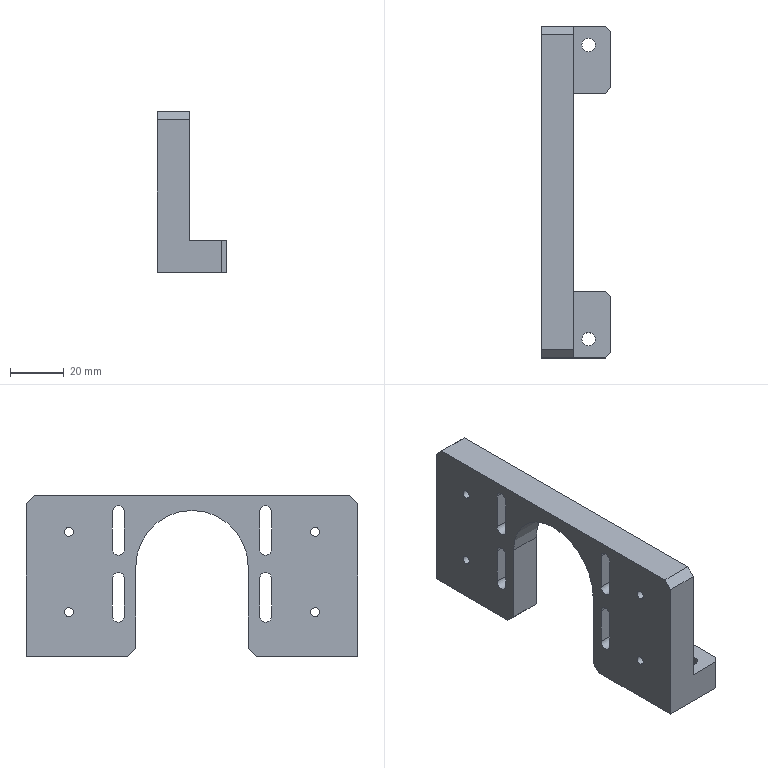Part | STEP file | 1 solid | 57 faces | box 26 x 124 x 60 mm | volume 67502 mm3 | plane 31 | cylinder 26 | commonest cylinder face diameters 4.5 x12 3.3 x8 5 x4 42 x2